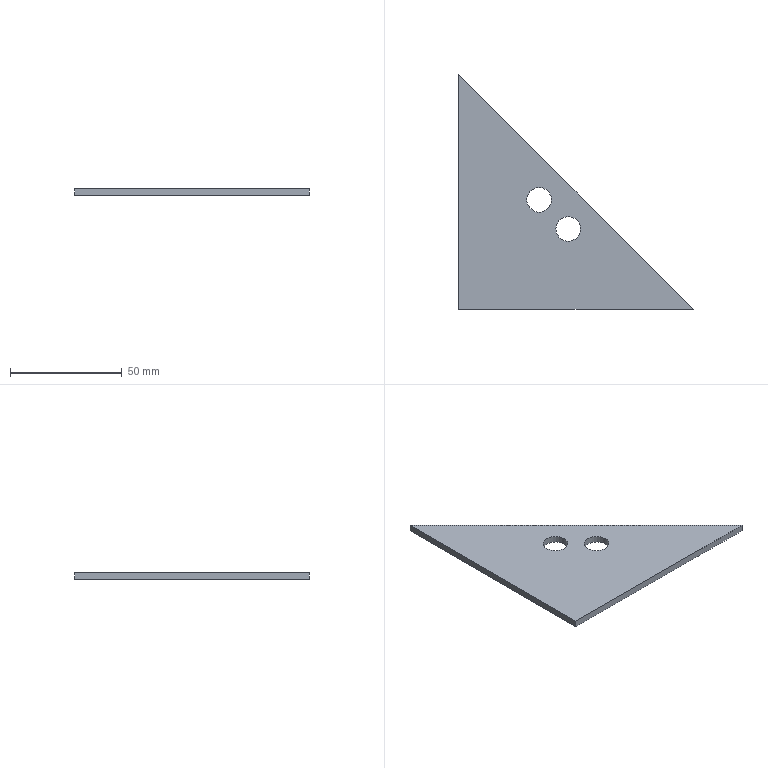Part | SolidWorks | features Cut 1, FlatPattern 1, SMBaseFlange 1, SheetMetal 1 | 1 solid | 9 faces | box 105 x 105 x 3 mm | volume 15967 mm3 | plane 5 | cylinder 4 | commonest cylinder face diameters 11 x4
STEP:
#1=CARTESIAN_POINT('',(30.5,49.,0.));
#2=VERTEX_POINT('',#1);
#3=CARTESIAN_POINT('',(41.5,49.,0.));
#4=VERTEX_POINT('',#3);
#5=CARTESIAN_POINT('',(36.,49.,0.));
#6=DIRECTION('',(0.,0.,1.));
#7=DIRECTION('',(1.,0.,0.));
#8=AXIS2_PLACEMENT_3D('',#5,#6,#7);
#9=CIRCLE('',#8,5.5);
#10=EDGE_CURVE('',#2,#4,#9,.T.);
#11=ORIENTED_EDGE('',*,*,#10,.T.);
#12=CARTESIAN_POINT('',(41.5,49.,-3.));
#13=VERTEX_POINT('',#12);
#14=CARTESIAN_POINT('',(41.5,49.,7.));
#15=DIRECTION('',(0.,0.,-1.));
#16=VECTOR('',#15,1000.);
#17=LINE('',#14,#16);
#18=EDGE_CURVE('',#4,#13,#17,.T.);
#19=ORIENTED_EDGE('',*,*,#18,.T.);
#20=CARTESIAN_POINT('',(30.5,49.,-3.));
#21=VERTEX_POINT('',#20);
#22=CARTESIAN_POINT('',(36.,49.,-3.));
#23=DIRECTION('',(0.,0.,-1.));
#24=DIRECTION('',(-1.,0.,0.));
#25=AXIS2_PLACEMENT_3D('',#22,#23,#24);
#26=CIRCLE('',#25,5.5);
#27=EDGE_CURVE('',#13,#21,#26,.T.);
#28=ORIENTED_EDGE('',*,*,#27,.T.);
#29=CARTESIAN_POINT('',(30.5,49.,7.));
#30=DIRECTION('',(0.,0.,-1.));
#31=VECTOR('',#30,1000.);
#32=LINE('',#29,#31);
#33=EDGE_CURVE('',#2,#21,#32,.T.);
#34=ORIENTED_EDGE('',*,*,#33,.F.);
#35=EDGE_LOOP('',(#11,#19,#28,#34));
#36=FACE_OUTER_BOUND('',#35,.T.);
#37=CARTESIAN_POINT('',(36.,49.,7.));
#38=DIRECTION('',(0.,0.,-1.));
#39=DIRECTION('',(-1.,0.,0.));
#40=AXIS2_PLACEMENT_3D('',#37,#38,#39);
#41=CYLINDRICAL_SURFACE('',#40,5.5);
#42=ADVANCED_FACE('',(#36),#41,.F.);
#43=CARTESIAN_POINT('',(43.5,36.,0.));
#44=VERTEX_POINT('',#43);
#45=CARTESIAN_POINT('',(54.5,36.,0.));
#46=VERTEX_POINT('',#45);
#47=CARTESIAN_POINT('',(49.,36.,0.));
#48=DIRECTION('',(0.,0.,1.));
#49=DIRECTION('',(1.,0.,0.));
#50=AXIS2_PLACEMENT_3D('',#47,#48,#49);
#51=CIRCLE('',#50,5.5);
#52=EDGE_CURVE('',#44,#46,#51,.T.);
#53=ORIENTED_EDGE('',*,*,#52,.T.);
#54=CARTESIAN_POINT('',(54.5,36.,-3.));
#55=VERTEX_POINT('',#54);
#56=CARTESIAN_POINT('',(54.5,36.,7.));
#57=DIRECTION('',(0.,0.,-1.));
#58=VECTOR('',#57,1000.);
#59=LINE('',#56,#58);
#60=EDGE_CURVE('',#46,#55,#59,.T.);
#61=ORIENTED_EDGE('',*,*,#60,.T.);
#62=CARTESIAN_POINT('',(43.5,36.,-3.));
#63=VERTEX_POINT('',#62);
#64=CARTESIAN_POINT('',(49.,36.,-3.));
#65=DIRECTION('',(0.,0.,-1.));
#66=DIRECTION('',(-1.,0.,0.));
#67=AXIS2_PLACEMENT_3D('',#64,#65,#66);
#68=CIRCLE('',#67,5.5);
#69=EDGE_CURVE('',#55,#63,#68,.T.);
#70=ORIENTED_EDGE('',*,*,#69,.T.);
#71=CARTESIAN_POINT('',(43.5,36.,7.));
#72=DIRECTION('',(0.,0.,-1.));
#73=VECTOR('',#72,1000.);
#74=LINE('',#71,#73);
#75=EDGE_CURVE('',#44,#63,#74,.T.);
#76=ORIENTED_EDGE('',*,*,#75,.F.);
#77=EDGE_LOOP('',(#53,#61,#70,#76));
#78=FACE_OUTER_BOUND('',#77,.T.);
#79=CARTESIAN_POINT('',(49.,36.,7.));
#80=DIRECTION('',(0.,0.,-1.));
#81=DIRECTION('',(-1.,0.,0.));
#82=AXIS2_PLACEMENT_3D('',#79,#80,#81);
#83=CYLINDRICAL_SURFACE('',#82,5.5);
#84=ADVANCED_FACE('',(#78),#83,.F.);
#85=CARTESIAN_POINT('',(0.,105.,0.));
#86=VERTEX_POINT('',#85);
#87=CARTESIAN_POINT('',(0.,0.,0.));
#88=VERTEX_POINT('',#87);
#89=CARTESIAN_POINT('',(0.,105.,0.));
#90=DIRECTION('',(0.,-1.,0.));
#91=VECTOR('',#90,1000.);
#92=LINE('',#89,#91);
#93=EDGE_CURVE('',#86,#88,#92,.T.);
#94=ORIENTED_EDGE('',*,*,#93,.F.);
#95=CARTESIAN_POINT('',(0.,105.,-3.));
#96=VERTEX_POINT('',#95);
#97=CARTESIAN_POINT('',(0.,105.,-3.));
#98=DIRECTION('',(0.,0.,1.));
#99=VECTOR('',#98,1000.);
#100=LINE('',#97,#99);
#101=EDGE_CURVE('',#96,#86,#100,.T.);
#102=ORIENTED_EDGE('',*,*,#101,.F.);
#103=CARTESIAN_POINT('',(0.,0.,-3.));
#104=VERTEX_POINT('',#103);
#105=CARTESIAN_POINT('',(0.,105.,-3.));
#106=DIRECTION('',(0.,-1.,0.));
#107=VECTOR('',#106,1000.);
#108=LINE('',#105,#107);
#109=EDGE_CURVE('',#96,#104,#108,.T.);
#110=ORIENTED_EDGE('',*,*,#109,.T.);
#111=CARTESIAN_POINT('',(0.,0.,-3.));
#112=DIRECTION('',(0.,0.,1.));
#113=VECTOR('',#112,1000.);
#114=LINE('',#111,#113);
#115=EDGE_CURVE('',#104,#88,#114,.T.);
#116=ORIENTED_EDGE('',*,*,#115,.T.);
#117=EDGE_LOOP('',(#94,#102,#110,#116));
#118=FACE_OUTER_BOUND('',#117,.T.);
#119=CARTESIAN_POINT('',(0.,105.,-3.));
#120=DIRECTION('',(-1.,0.,0.));
#121=DIRECTION('',(0.,-1.,0.));
#122=AXIS2_PLACEMENT_3D('',#119,#120,#121);
#123=PLANE('',#122);
#124=ADVANCED_FACE('',(#118),#123,.T.);
#125=CARTESIAN_POINT('',(105.,0.,0.));
#126=VERTEX_POINT('',#125);
#127=CARTESIAN_POINT('',(105.,0.,0.));
#128=DIRECTION('',(-0.7071,0.7071,0.));
#129=VECTOR('',#128,1000.);
#130=LINE('',#127,#129);
#131=EDGE_CURVE('',#126,#86,#130,.T.);
#132=ORIENTED_EDGE('',*,*,#131,.F.);
#133=CARTESIAN_POINT('',(105.,0.,-3.));
#134=VERTEX_POINT('',#133);
#135=CARTESIAN_POINT('',(105.,0.,-3.));
#136=DIRECTION('',(0.,0.,1.));
#137=VECTOR('',#136,1000.);
#138=LINE('',#135,#137);
#139=EDGE_CURVE('',#134,#126,#138,.T.);
#140=ORIENTED_EDGE('',*,*,#139,.F.);
#141=CARTESIAN_POINT('',(105.,0.,-3.));
#142=DIRECTION('',(-0.7071,0.7071,0.));
#143=VECTOR('',#142,1000.);
#144=LINE('',#141,#143);
#145=EDGE_CURVE('',#134,#96,#144,.T.);
#146=ORIENTED_EDGE('',*,*,#145,.T.);
#147=ORIENTED_EDGE('',*,*,#101,.T.);
#148=EDGE_LOOP('',(#132,#140,#146,#147));
#149=FACE_OUTER_BOUND('',#148,.T.);
#150=CARTESIAN_POINT('',(105.,0.,-3.));
#151=DIRECTION('',(0.7071,0.7071,0.));
#152=DIRECTION('',(-0.7071,0.7071,0.));
#153=AXIS2_PLACEMENT_3D('',#150,#151,#152);
#154=PLANE('',#153);
#155=ADVANCED_FACE('',(#149),#154,.T.);
#156=CARTESIAN_POINT('',(0.,0.,0.));
#157=DIRECTION('',(1.,0.,0.));
#158=VECTOR('',#157,1000.);
#159=LINE('',#156,#158);
#160=EDGE_CURVE('',#88,#126,#159,.T.);
#161=ORIENTED_EDGE('',*,*,#160,.F.);
#162=ORIENTED_EDGE('',*,*,#115,.F.);
#163=CARTESIAN_POINT('',(0.,0.,-3.));
#164=DIRECTION('',(1.,0.,0.));
#165=VECTOR('',#164,1000.);
#166=LINE('',#163,#165);
#167=EDGE_CURVE('',#104,#134,#166,.T.);
#168=ORIENTED_EDGE('',*,*,#167,.T.);
#169=ORIENTED_EDGE('',*,*,#139,.T.);
#170=EDGE_LOOP('',(#161,#162,#168,#169));
#171=FACE_OUTER_BOUND('',#170,.T.);
#172=CARTESIAN_POINT('',(0.,0.,-3.));
#173=DIRECTION('',(0.,-1.,0.));
#174=DIRECTION('',(1.,0.,0.));
#175=AXIS2_PLACEMENT_3D('',#172,#173,#174);
#176=PLANE('',#175);
#177=ADVANCED_FACE('',(#171),#176,.T.);
#178=CARTESIAN_POINT('',(36.,49.,-3.));
#179=DIRECTION('',(0.,0.,-1.));
#180=DIRECTION('',(-1.,0.,0.));
#181=AXIS2_PLACEMENT_3D('',#178,#179,#180);
#182=CIRCLE('',#181,5.5);
#183=EDGE_CURVE('',#21,#13,#182,.T.);
#184=ORIENTED_EDGE('',*,*,#183,.F.);
#185=ORIENTED_EDGE('',*,*,#27,.F.);
#186=EDGE_LOOP('',(#184,#185));
#187=FACE_BOUND('',#186,.T.);
#188=CARTESIAN_POINT('',(49.,36.,-3.));
#189=DIRECTION('',(0.,0.,-1.));
#190=DIRECTION('',(-1.,0.,0.));
#191=AXIS2_PLACEMENT_3D('',#188,#189,#190);
#192=CIRCLE('',#191,5.5);
#193=EDGE_CURVE('',#63,#55,#192,.T.);
#194=ORIENTED_EDGE('',*,*,#193,.F.);
#195=ORIENTED_EDGE('',*,*,#69,.F.);
#196=EDGE_LOOP('',(#194,#195));
#197=FACE_BOUND('',#196,.T.);
#198=ORIENTED_EDGE('',*,*,#109,.F.);
#199=ORIENTED_EDGE('',*,*,#145,.F.);
#200=ORIENTED_EDGE('',*,*,#167,.F.);
#201=EDGE_LOOP('',(#198,#199,#200));
#202=FACE_OUTER_BOUND('',#201,.T.);
#203=CARTESIAN_POINT('',(0.,0.,-3.));
#204=DIRECTION('',(0.,0.,1.));
#205=DIRECTION('',(1.,0.,0.));
#206=AXIS2_PLACEMENT_3D('',#203,#204,#205);
#207=PLANE('',#206);
#208=ADVANCED_FACE('',(#187,#197,#202),#207,.F.);
#209=ORIENTED_EDGE('',*,*,#10,.F.);
#210=CARTESIAN_POINT('',(36.,49.,0.));
#211=DIRECTION('',(0.,0.,1.));
#212=DIRECTION('',(1.,0.,0.));
#213=AXIS2_PLACEMENT_3D('',#210,#211,#212);
#214=CIRCLE('',#213,5.5);
#215=EDGE_CURVE('',#4,#2,#214,.T.);
#216=ORIENTED_EDGE('',*,*,#215,.F.);
#217=EDGE_LOOP('',(#209,#216));
#218=FACE_BOUND('',#217,.T.);
#219=ORIENTED_EDGE('',*,*,#52,.F.);
#220=CARTESIAN_POINT('',(49.,36.,0.));
#221=DIRECTION('',(0.,0.,1.));
#222=DIRECTION('',(1.,0.,0.));
#223=AXIS2_PLACEMENT_3D('',#220,#221,#222);
#224=CIRCLE('',#223,5.5);
#225=EDGE_CURVE('',#46,#44,#224,.T.);
#226=ORIENTED_EDGE('',*,*,#225,.F.);
#227=EDGE_LOOP('',(#219,#226));
#228=FACE_BOUND('',#227,.T.);
#229=ORIENTED_EDGE('',*,*,#93,.T.);
#230=ORIENTED_EDGE('',*,*,#160,.T.);
#231=ORIENTED_EDGE('',*,*,#131,.T.);
#232=EDGE_LOOP('',(#229,#230,#231));
#233=FACE_OUTER_BOUND('',#232,.T.);
#234=CARTESIAN_POINT('',(0.,0.,0.));
#235=DIRECTION('',(0.,0.,1.));
#236=DIRECTION('',(1.,0.,0.));
#237=AXIS2_PLACEMENT_3D('',#234,#235,#236);
#238=PLANE('',#237);
#239=ADVANCED_FACE('',(#218,#228,#233),#238,.T.);
#240=ORIENTED_EDGE('',*,*,#60,.F.);
#241=ORIENTED_EDGE('',*,*,#225,.T.);
#242=ORIENTED_EDGE('',*,*,#75,.T.);
#243=ORIENTED_EDGE('',*,*,#193,.T.);
#244=EDGE_LOOP('',(#240,#241,#242,#243));
#245=FACE_OUTER_BOUND('',#244,.T.);
#246=CARTESIAN_POINT('',(49.,36.,7.));
#247=DIRECTION('',(0.,0.,-1.));
#248=DIRECTION('',(-1.,0.,0.));
#249=AXIS2_PLACEMENT_3D('',#246,#247,#248);
#250=CYLINDRICAL_SURFACE('',#249,5.5);
#251=ADVANCED_FACE('',(#245),#250,.F.);
#252=ORIENTED_EDGE('',*,*,#18,.F.);
#253=ORIENTED_EDGE('',*,*,#215,.T.);
#254=ORIENTED_EDGE('',*,*,#33,.T.);
#255=ORIENTED_EDGE('',*,*,#183,.T.);
#256=EDGE_LOOP('',(#252,#253,#254,#255));
#257=FACE_OUTER_BOUND('',#256,.T.);
#258=CARTESIAN_POINT('',(36.,49.,7.));
#259=DIRECTION('',(0.,0.,-1.));
#260=DIRECTION('',(-1.,0.,0.));
#261=AXIS2_PLACEMENT_3D('',#258,#259,#260);
#262=CYLINDRICAL_SURFACE('',#261,5.5);
#263=ADVANCED_FACE('',(#257),#262,.F.);
#264=CLOSED_SHELL('',(#42,#84,#124,#155,#177,#208,#239,#251,#263));
#265=MANIFOLD_SOLID_BREP('',#264);
#266=CARTESIAN_POINT('',(0.,0.,0.));
#267=DIRECTION('',(0.,0.,1.));
#268=DIRECTION('',(1.,0.,0.));
#269=AXIS2_PLACEMENT_3D('',#266,#267,#268);
#270=(LENGTH_UNIT()NAMED_UNIT(*)SI_UNIT(.MILLI.,.METRE.));
#271=UNCERTAINTY_MEASURE_WITH_UNIT(LENGTH_MEASURE(0.00001),#270,'','');
#272=(NAMED_UNIT(*)PLANE_ANGLE_UNIT()SI_UNIT($,.RADIAN.));
#273=(NAMED_UNIT(*)SI_UNIT($,.STERADIAN.)SOLID_ANGLE_UNIT());
#274=(GEOMETRIC_REPRESENTATION_CONTEXT(3)GLOBAL_UNCERTAINTY_ASSIGNED_CONTEXT((#271))GLOBAL_UNIT_ASSIGNED_CONTEXT((#270,#272,#273))REPRESENTATION_CONTEXT('',''));
#275=ADVANCED_BREP_SHAPE_REPRESENTATION('',(#265,#269),#274);